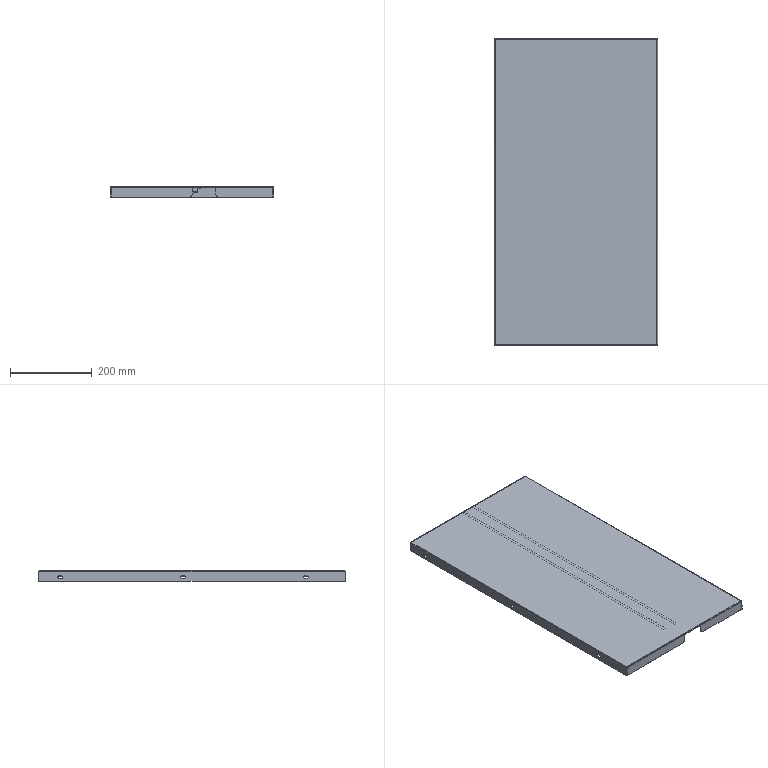Part | STEP file | FBDS-BJ-003 | 2 solids | 122 faces | box 398 x 748 x 25 mm | volume 585293 mm3 | plane 80 | cylinder 34 | spline 8 | commonest cylinder face diameters 6.5 x16 0.4 x8 3.4 x8 20 x2